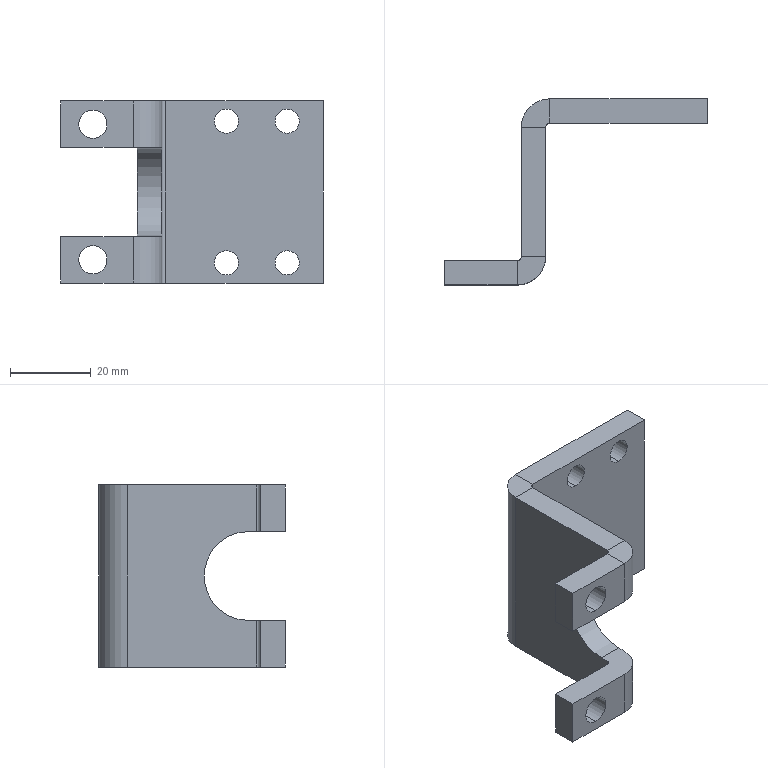Part | SolidWorks | features ICE 3, FlatPattern 1, SMBaseFlange 1, SheetMetal 1 | 1 solid | 42 faces | box 65 x 46 x 45 mm | volume 21673 mm3 | plane 23 | cylinder 19 | commonest cylinder face diameters 6 x8 7 x4 2 x3 14 x3 22 x1
STEP:
#1=CARTESIAN_POINT('',(8.,0.,2.25));
#2=VERTEX_POINT('',#1);
#3=CARTESIAN_POINT('',(8.,0.,9.25));
#4=VERTEX_POINT('',#3);
#5=CARTESIAN_POINT('',(8.,0.,5.75));
#6=DIRECTION('',(0.,1.,0.));
#7=DIRECTION('',(0.,0.,1.));
#8=AXIS2_PLACEMENT_3D('',#5,#6,#7);
#9=CIRCLE('',#8,3.5);
#10=EDGE_CURVE('',#2,#4,#9,.T.);
#11=ORIENTED_EDGE('',*,*,#10,.F.);
#12=CARTESIAN_POINT('',(8.,6.,2.25));
#13=VERTEX_POINT('',#12);
#14=CARTESIAN_POINT('',(8.,-4.,2.25));
#15=DIRECTION('',(0.,1.,0.));
#16=VECTOR('',#15,1000.);
#17=LINE('',#14,#16);
#18=EDGE_CURVE('',#2,#13,#17,.T.);
#19=ORIENTED_EDGE('',*,*,#18,.T.);
#20=CARTESIAN_POINT('',(8.,6.,9.25));
#21=VERTEX_POINT('',#20);
#22=CARTESIAN_POINT('',(8.,6.,5.75));
#23=DIRECTION('',(0.,1.,0.));
#24=DIRECTION('',(0.,0.,1.));
#25=AXIS2_PLACEMENT_3D('',#22,#23,#24);
#26=CIRCLE('',#25,3.5);
#27=EDGE_CURVE('',#13,#21,#26,.T.);
#28=ORIENTED_EDGE('',*,*,#27,.T.);
#29=CARTESIAN_POINT('',(8.,-4.,9.25));
#30=DIRECTION('',(0.,1.,0.));
#31=VECTOR('',#30,1000.);
#32=LINE('',#29,#31);
#33=EDGE_CURVE('',#4,#21,#32,.T.);
#34=ORIENTED_EDGE('',*,*,#33,.F.);
#35=EDGE_LOOP('',(#11,#19,#28,#34));
#36=FACE_OUTER_BOUND('',#35,.T.);
#37=CARTESIAN_POINT('',(8.,-4.,5.75));
#38=DIRECTION('',(0.,1.,0.));
#39=DIRECTION('',(0.,0.,1.));
#40=AXIS2_PLACEMENT_3D('',#37,#38,#39);
#41=CYLINDRICAL_SURFACE('',#40,3.5);
#42=ADVANCED_FACE('',(#36),#41,.F.);
#43=CARTESIAN_POINT('',(8.,0.,35.75));
#44=VERTEX_POINT('',#43);
#45=CARTESIAN_POINT('',(8.,0.,42.75));
#46=VERTEX_POINT('',#45);
#47=CARTESIAN_POINT('',(8.,0.,39.25));
#48=DIRECTION('',(0.,1.,0.));
#49=DIRECTION('',(0.,0.,1.));
#50=AXIS2_PLACEMENT_3D('',#47,#48,#49);
#51=CIRCLE('',#50,3.5);
#52=EDGE_CURVE('',#44,#46,#51,.T.);
#53=ORIENTED_EDGE('',*,*,#52,.F.);
#54=CARTESIAN_POINT('',(8.,6.,35.75));
#55=VERTEX_POINT('',#54);
#56=CARTESIAN_POINT('',(8.,-4.,35.75));
#57=DIRECTION('',(0.,1.,0.));
#58=VECTOR('',#57,1000.);
#59=LINE('',#56,#58);
#60=EDGE_CURVE('',#44,#55,#59,.T.);
#61=ORIENTED_EDGE('',*,*,#60,.T.);
#62=CARTESIAN_POINT('',(8.,6.,42.75));
#63=VERTEX_POINT('',#62);
#64=CARTESIAN_POINT('',(8.,6.,39.25));
#65=DIRECTION('',(0.,1.,0.));
#66=DIRECTION('',(0.,0.,1.));
#67=AXIS2_PLACEMENT_3D('',#64,#65,#66);
#68=CIRCLE('',#67,3.5);
#69=EDGE_CURVE('',#55,#63,#68,.T.);
#70=ORIENTED_EDGE('',*,*,#69,.T.);
#71=CARTESIAN_POINT('',(8.,-4.,42.75));
#72=DIRECTION('',(0.,1.,0.));
#73=VECTOR('',#72,1000.);
#74=LINE('',#71,#73);
#75=EDGE_CURVE('',#46,#63,#74,.T.);
#76=ORIENTED_EDGE('',*,*,#75,.F.);
#77=EDGE_LOOP('',(#53,#61,#70,#76));
#78=FACE_OUTER_BOUND('',#77,.T.);
#79=CARTESIAN_POINT('',(8.,-4.,39.25));
#80=DIRECTION('',(0.,1.,0.));
#81=DIRECTION('',(0.,0.,1.));
#82=AXIS2_PLACEMENT_3D('',#79,#80,#81);
#83=CYLINDRICAL_SURFACE('',#82,3.5);
#84=ADVANCED_FACE('',(#78),#83,.F.);
#85=CARTESIAN_POINT('',(56.,40.,2.));
#86=VERTEX_POINT('',#85);
#87=CARTESIAN_POINT('',(56.,40.,8.));
#88=VERTEX_POINT('',#87);
#89=CARTESIAN_POINT('',(56.,40.,5.));
#90=DIRECTION('',(0.,1.,0.));
#91=DIRECTION('',(0.,0.,1.));
#92=AXIS2_PLACEMENT_3D('',#89,#90,#91);
#93=CIRCLE('',#92,3.);
#94=EDGE_CURVE('',#86,#88,#93,.T.);
#95=ORIENTED_EDGE('',*,*,#94,.F.);
#96=CARTESIAN_POINT('',(56.,46.,2.));
#97=VERTEX_POINT('',#96);
#98=CARTESIAN_POINT('',(56.,36.,2.));
#99=DIRECTION('',(0.,1.,0.));
#100=VECTOR('',#99,1000.);
#101=LINE('',#98,#100);
#102=EDGE_CURVE('',#86,#97,#101,.T.);
#103=ORIENTED_EDGE('',*,*,#102,.T.);
#104=CARTESIAN_POINT('',(56.,46.,8.));
#105=VERTEX_POINT('',#104);
#106=CARTESIAN_POINT('',(56.,46.,5.));
#107=DIRECTION('',(0.,1.,0.));
#108=DIRECTION('',(0.,0.,1.));
#109=AXIS2_PLACEMENT_3D('',#106,#107,#108);
#110=CIRCLE('',#109,3.);
#111=EDGE_CURVE('',#97,#105,#110,.T.);
#112=ORIENTED_EDGE('',*,*,#111,.T.);
#113=CARTESIAN_POINT('',(56.,36.,8.));
#114=DIRECTION('',(0.,1.,0.));
#115=VECTOR('',#114,1000.);
#116=LINE('',#113,#115);
#117=EDGE_CURVE('',#88,#105,#116,.T.);
#118=ORIENTED_EDGE('',*,*,#117,.F.);
#119=EDGE_LOOP('',(#95,#103,#112,#118));
#120=FACE_OUTER_BOUND('',#119,.T.);
#121=CARTESIAN_POINT('',(56.,36.,5.));
#122=DIRECTION('',(0.,1.,0.));
#123=DIRECTION('',(0.,0.,1.));
#124=AXIS2_PLACEMENT_3D('',#121,#122,#123);
#125=CYLINDRICAL_SURFACE('',#124,3.);
#126=ADVANCED_FACE('',(#120),#125,.F.);
#127=CARTESIAN_POINT('',(56.,40.,37.));
#128=VERTEX_POINT('',#127);
#129=CARTESIAN_POINT('',(56.,40.,43.));
#130=VERTEX_POINT('',#129);
#131=CARTESIAN_POINT('',(56.,40.,40.));
#132=DIRECTION('',(0.,1.,0.));
#133=DIRECTION('',(0.,0.,1.));
#134=AXIS2_PLACEMENT_3D('',#131,#132,#133);
#135=CIRCLE('',#134,3.);
#136=EDGE_CURVE('',#128,#130,#135,.T.);
#137=ORIENTED_EDGE('',*,*,#136,.F.);
#138=CARTESIAN_POINT('',(56.,46.,37.));
#139=VERTEX_POINT('',#138);
#140=CARTESIAN_POINT('',(56.,36.,37.));
#141=DIRECTION('',(0.,1.,0.));
#142=VECTOR('',#141,1000.);
#143=LINE('',#140,#142);
#144=EDGE_CURVE('',#128,#139,#143,.T.);
#145=ORIENTED_EDGE('',*,*,#144,.T.);
#146=CARTESIAN_POINT('',(56.,46.,43.));
#147=VERTEX_POINT('',#146);
#148=CARTESIAN_POINT('',(56.,46.,40.));
#149=DIRECTION('',(0.,1.,0.));
#150=DIRECTION('',(0.,0.,1.));
#151=AXIS2_PLACEMENT_3D('',#148,#149,#150);
#152=CIRCLE('',#151,3.);
#153=EDGE_CURVE('',#139,#147,#152,.T.);
#154=ORIENTED_EDGE('',*,*,#153,.T.);
#155=CARTESIAN_POINT('',(56.,36.,43.));
#156=DIRECTION('',(0.,1.,0.));
#157=VECTOR('',#156,1000.);
#158=LINE('',#155,#157);
#159=EDGE_CURVE('',#130,#147,#158,.T.);
#160=ORIENTED_EDGE('',*,*,#159,.F.);
#161=EDGE_LOOP('',(#137,#145,#154,#160));
#162=FACE_OUTER_BOUND('',#161,.T.);
#163=CARTESIAN_POINT('',(56.,36.,40.));
#164=DIRECTION('',(0.,1.,0.));
#165=DIRECTION('',(0.,0.,1.));
#166=AXIS2_PLACEMENT_3D('',#163,#164,#165);
#167=CYLINDRICAL_SURFACE('',#166,3.);
#168=ADVANCED_FACE('',(#162),#167,.F.);
#169=CARTESIAN_POINT('',(41.,40.,37.));
#170=VERTEX_POINT('',#169);
#171=CARTESIAN_POINT('',(41.,40.,43.));
#172=VERTEX_POINT('',#171);
#173=CARTESIAN_POINT('',(41.,40.,40.));
#174=DIRECTION('',(0.,1.,0.));
#175=DIRECTION('',(0.,0.,1.));
#176=AXIS2_PLACEMENT_3D('',#173,#174,#175);
#177=CIRCLE('',#176,3.);
#178=EDGE_CURVE('',#170,#172,#177,.T.);
#179=ORIENTED_EDGE('',*,*,#178,.F.);
#180=CARTESIAN_POINT('',(41.,46.,37.));
#181=VERTEX_POINT('',#180);
#182=CARTESIAN_POINT('',(41.,36.,37.));
#183=DIRECTION('',(0.,1.,0.));
#184=VECTOR('',#183,1000.);
#185=LINE('',#182,#184);
#186=EDGE_CURVE('',#170,#181,#185,.T.);
#187=ORIENTED_EDGE('',*,*,#186,.T.);
#188=CARTESIAN_POINT('',(41.,46.,43.));
#189=VERTEX_POINT('',#188);
#190=CARTESIAN_POINT('',(41.,46.,40.));
#191=DIRECTION('',(0.,1.,0.));
#192=DIRECTION('',(0.,0.,1.));
#193=AXIS2_PLACEMENT_3D('',#190,#191,#192);
#194=CIRCLE('',#193,3.);
#195=EDGE_CURVE('',#181,#189,#194,.T.);
#196=ORIENTED_EDGE('',*,*,#195,.T.);
#197=CARTESIAN_POINT('',(41.,36.,43.));
#198=DIRECTION('',(0.,1.,0.));
#199=VECTOR('',#198,1000.);
#200=LINE('',#197,#199);
#201=EDGE_CURVE('',#172,#189,#200,.T.);
#202=ORIENTED_EDGE('',*,*,#201,.F.);
#203=EDGE_LOOP('',(#179,#187,#196,#202));
#204=FACE_OUTER_BOUND('',#203,.T.);
#205=CARTESIAN_POINT('',(41.,36.,40.));
#206=DIRECTION('',(0.,1.,0.));
#207=DIRECTION('',(0.,0.,1.));
#208=AXIS2_PLACEMENT_3D('',#205,#206,#207);
#209=CYLINDRICAL_SURFACE('',#208,3.);
#210=ADVANCED_FACE('',(#204),#209,.F.);
#211=CARTESIAN_POINT('',(41.,40.,2.));
#212=VERTEX_POINT('',#211);
#213=CARTESIAN_POINT('',(41.,40.,8.));
#214=VERTEX_POINT('',#213);
#215=CARTESIAN_POINT('',(41.,40.,5.));
#216=DIRECTION('',(0.,1.,0.));
#217=DIRECTION('',(0.,0.,1.));
#218=AXIS2_PLACEMENT_3D('',#215,#216,#217);
#219=CIRCLE('',#218,3.);
#220=EDGE_CURVE('',#212,#214,#219,.T.);
#221=ORIENTED_EDGE('',*,*,#220,.F.);
#222=CARTESIAN_POINT('',(41.,46.,2.));
#223=VERTEX_POINT('',#222);
#224=CARTESIAN_POINT('',(41.,36.,2.));
#225=DIRECTION('',(0.,1.,0.));
#226=VECTOR('',#225,1000.);
#227=LINE('',#224,#226);
#228=EDGE_CURVE('',#212,#223,#227,.T.);
#229=ORIENTED_EDGE('',*,*,#228,.T.);
#230=CARTESIAN_POINT('',(41.,46.,8.));
#231=VERTEX_POINT('',#230);
#232=CARTESIAN_POINT('',(41.,46.,5.));
#233=DIRECTION('',(0.,1.,0.));
#234=DIRECTION('',(0.,0.,1.));
#235=AXIS2_PLACEMENT_3D('',#232,#233,#234);
#236=CIRCLE('',#235,3.);
#237=EDGE_CURVE('',#223,#231,#236,.T.);
#238=ORIENTED_EDGE('',*,*,#237,.T.);
#239=CARTESIAN_POINT('',(41.,36.,8.));
#240=DIRECTION('',(0.,1.,0.));
#241=VECTOR('',#240,1000.);
#242=LINE('',#239,#241);
#243=EDGE_CURVE('',#214,#231,#242,.T.);
#244=ORIENTED_EDGE('',*,*,#243,.F.);
#245=EDGE_LOOP('',(#221,#229,#238,#244));
#246=FACE_OUTER_BOUND('',#245,.T.);
#247=CARTESIAN_POINT('',(41.,36.,5.));
#248=DIRECTION('',(0.,1.,0.));
#249=DIRECTION('',(0.,0.,1.));
#250=AXIS2_PLACEMENT_3D('',#247,#248,#249);
#251=CYLINDRICAL_SURFACE('',#250,3.);
#252=ADVANCED_FACE('',(#246),#251,.F.);
#253=CARTESIAN_POINT('',(19.,7.,11.5));
#254=VERTEX_POINT('',#253);
#255=CARTESIAN_POINT('',(18.,6.,11.5));
#256=VERTEX_POINT('',#255);
#257=CARTESIAN_POINT('',(18.,7.,11.5));
#258=DIRECTION('',(0.,0.,-1.));
#259=DIRECTION('',(-1.,0.,0.));
#260=AXIS2_PLACEMENT_3D('',#257,#258,#259);
#261=CIRCLE('',#260,1.);
#262=EDGE_CURVE('',#254,#256,#261,.T.);
#263=ORIENTED_EDGE('',*,*,#262,.F.);
#264=CARTESIAN_POINT('',(19.,7.,0.));
#265=VERTEX_POINT('',#264);
#266=CARTESIAN_POINT('',(19.,7.,45.));
#267=DIRECTION('',(0.,0.,-1.));
#268=VECTOR('',#267,1000.);
#269=LINE('',#266,#268);
#270=EDGE_CURVE('',#254,#265,#269,.T.);
#271=ORIENTED_EDGE('',*,*,#270,.T.);
#272=CARTESIAN_POINT('',(18.,6.,0.));
#273=VERTEX_POINT('',#272);
#274=CARTESIAN_POINT('',(18.,7.,0.));
#275=DIRECTION('',(0.,0.,1.));
#276=DIRECTION('',(1.,0.,0.));
#277=AXIS2_PLACEMENT_3D('',#274,#275,#276);
#278=CIRCLE('',#277,1.);
#279=EDGE_CURVE('',#273,#265,#278,.T.);
#280=ORIENTED_EDGE('',*,*,#279,.F.);
#281=CARTESIAN_POINT('',(18.,6.,45.));
#282=DIRECTION('',(0.,0.,-1.));
#283=VECTOR('',#282,1000.);
#284=LINE('',#281,#283);
#285=EDGE_CURVE('',#256,#273,#284,.T.);
#286=ORIENTED_EDGE('',*,*,#285,.F.);
#287=EDGE_LOOP('',(#263,#271,#280,#286));
#288=FACE_OUTER_BOUND('',#287,.T.);
#289=CARTESIAN_POINT('',(18.,7.,45.));
#290=DIRECTION('',(0.,0.,-1.));
#291=DIRECTION('',(-1.,0.,0.));
#292=AXIS2_PLACEMENT_3D('',#289,#290,#291);
#293=CYLINDRICAL_SURFACE('',#292,1.);
#294=ADVANCED_FACE('',(#288),#293,.F.);
#295=CARTESIAN_POINT('',(8.,6.,5.75));
#296=DIRECTION('',(0.,1.,0.));
#297=DIRECTION('',(0.,0.,1.));
#298=AXIS2_PLACEMENT_3D('',#295,#296,#297);
#299=CIRCLE('',#298,3.5);
#300=EDGE_CURVE('',#21,#13,#299,.T.);
#301=ORIENTED_EDGE('',*,*,#300,.F.);
#302=ORIENTED_EDGE('',*,*,#27,.F.);
#303=EDGE_LOOP('',(#301,#302));
#304=FACE_BOUND('',#303,.T.);
#305=CARTESIAN_POINT('',(0.,6.,11.5));
#306=VERTEX_POINT('',#305);
#307=CARTESIAN_POINT('',(0.,6.,11.5));
#308=DIRECTION('',(-1.,0.,0.));
#309=VECTOR('',#308,1000.);
#310=LINE('',#307,#309);
#311=EDGE_CURVE('',#256,#306,#310,.T.);
#312=ORIENTED_EDGE('',*,*,#311,.F.);
#313=ORIENTED_EDGE('',*,*,#285,.T.);
#314=CARTESIAN_POINT('',(0.,6.,0.));
#315=VERTEX_POINT('',#314);
#316=CARTESIAN_POINT('',(0.,6.,0.));
#317=DIRECTION('',(1.,0.,0.));
#318=VECTOR('',#317,1000.);
#319=LINE('',#316,#318);
#320=EDGE_CURVE('',#315,#273,#319,.T.);
#321=ORIENTED_EDGE('',*,*,#320,.F.);
#322=CARTESIAN_POINT('',(0.,6.,45.));
#323=DIRECTION('',(0.,0.,-1.));
#324=VECTOR('',#323,1000.);
#325=LINE('',#322,#324);
#326=EDGE_CURVE('',#306,#315,#325,.T.);
#327=ORIENTED_EDGE('',*,*,#326,.F.);
#328=EDGE_LOOP('',(#312,#313,#321,#327));
#329=FACE_OUTER_BOUND('',#328,.T.);
#330=CARTESIAN_POINT('',(0.,6.,45.));
#331=DIRECTION('',(0.,1.,0.));
#332=DIRECTION('',(0.,0.,1.));
#333=AXIS2_PLACEMENT_3D('',#330,#331,#332);
#334=PLANE('',#333);
#335=ADVANCED_FACE('',(#304,#329),#334,.T.);
#336=CARTESIAN_POINT('',(0.,0.,11.5));
#337=VERTEX_POINT('',#336);
#338=CARTESIAN_POINT('',(0.,-9.188,11.5));
#339=DIRECTION('',(0.,-1.,0.));
#340=VECTOR('',#339,1000.);
#341=LINE('',#338,#340);
#342=EDGE_CURVE('',#306,#337,#341,.T.);
#343=ORIENTED_EDGE('',*,*,#342,.F.);
#344=ORIENTED_EDGE('',*,*,#326,.T.);
#345=CARTESIAN_POINT('',(0.,0.,0.));
#346=VERTEX_POINT('',#345);
#347=CARTESIAN_POINT('',(0.,0.,0.));
#348=DIRECTION('',(0.,1.,0.));
#349=VECTOR('',#348,1000.);
#350=LINE('',#347,#349);
#351=EDGE_CURVE('',#346,#315,#350,.T.);
#352=ORIENTED_EDGE('',*,*,#351,.F.);
#353=CARTESIAN_POINT('',(0.,0.,45.));
#354=DIRECTION('',(0.,0.,-1.));
#355=VECTOR('',#354,1000.);
#356=LINE('',#353,#355);
#357=EDGE_CURVE('',#337,#346,#356,.T.);
#358=ORIENTED_EDGE('',*,*,#357,.F.);
#359=EDGE_LOOP('',(#343,#344,#352,#358));
#360=FACE_OUTER_BOUND('',#359,.T.);
#361=CARTESIAN_POINT('',(0.,0.,45.));
#362=DIRECTION('',(-1.,0.,0.));
#363=DIRECTION('',(0.,0.,1.));
#364=AXIS2_PLACEMENT_3D('',#361,#362,#363);
#365=PLANE('',#364);
#366=ADVANCED_FACE('',(#360),#365,.T.);
#367=CARTESIAN_POINT('',(8.,0.,5.75));
#368=DIRECTION('',(0.,1.,0.));
#369=DIRECTION('',(0.,0.,1.));
#370=AXIS2_PLACEMENT_3D('',#367,#368,#369);
#371=CIRCLE('',#370,3.5);
#372=EDGE_CURVE('',#4,#2,#371,.T.);
#373=ORIENTED_EDGE('',*,*,#372,.T.);
#374=ORIENTED_EDGE('',*,*,#10,.T.);
#375=EDGE_LOOP('',(#373,#374));
#376=FACE_BOUND('',#375,.T.);
#377=CARTESIAN_POINT('',(18.,0.,11.5));
#378=VERTEX_POINT('',#377);
#379=CARTESIAN_POINT('',(18.,0.,0.));
#380=VERTEX_POINT('',#379);
#381=CARTESIAN_POINT('',(18.,0.,45.));
#382=DIRECTION('',(0.,0.,-1.));
#383=VECTOR('',#382,1000.);
#384=LINE('',#381,#383);
#385=EDGE_CURVE('',#378,#380,#384,.T.);
#386=ORIENTED_EDGE('',*,*,#385,.F.);
#387=CARTESIAN_POINT('',(0.,0.,11.5));
#388=DIRECTION('',(-1.,0.,0.));
#389=VECTOR('',#388,1000.);
#390=LINE('',#387,#389);
#391=EDGE_CURVE('',#378,#337,#390,.T.);
#392=ORIENTED_EDGE('',*,*,#391,.T.);
#393=ORIENTED_EDGE('',*,*,#357,.T.);
#394=CARTESIAN_POINT('',(0.,0.,0.));
#395=DIRECTION('',(1.,0.,0.));
#396=VECTOR('',#395,1000.);
#397=LINE('',#394,#396);
#398=EDGE_CURVE('',#346,#380,#397,.T.);
#399=ORIENTED_EDGE('',*,*,#398,.T.);
#400=EDGE_LOOP('',(#386,#392,#393,#399));
#401=FACE_OUTER_BOUND('',#400,.T.);
#402=CARTESIAN_POINT('',(0.,0.,45.));
#403=DIRECTION('',(0.,1.,0.));
#404=DIRECTION('',(0.,0.,1.));
#405=AXIS2_PLACEMENT_3D('',#402,#403,#404);
#406=PLANE('',#405);
#407=ADVANCED_FACE('',(#376,#401),#406,.F.);
#408=CARTESIAN_POINT('',(25.,7.,11.5));
#409=VERTEX_POINT('',#408);
#410=CARTESIAN_POINT('',(25.,7.,0.));
#411=VERTEX_POINT('',#410);
#412=CARTESIAN_POINT('',(25.,7.,45.));
#413=DIRECTION('',(0.,0.,-1.));
#414=VECTOR('',#413,1000.);
#415=LINE('',#412,#414);
#416=EDGE_CURVE('',#409,#411,#415,.T.);
#417=ORIENTED_EDGE('',*,*,#416,.F.);
#418=CARTESIAN_POINT('',(18.,7.,11.5));
#419=DIRECTION('',(0.,0.,-1.));
#420=DIRECTION('',(-1.,0.,0.));
#421=AXIS2_PLACEMENT_3D('',#418,#419,#420);
#422=CIRCLE('',#421,7.);
#423=EDGE_CURVE('',#409,#378,#422,.T.);
#424=ORIENTED_EDGE('',*,*,#423,.T.);
#425=ORIENTED_EDGE('',*,*,#385,.T.);
#426=CARTESIAN_POINT('',(18.,7.,0.));
#427=DIRECTION('',(0.,0.,1.));
#428=DIRECTION('',(-1.,0.,0.));
#429=AXIS2_PLACEMENT_3D('',#426,#427,#428);
#430=CIRCLE('',#429,7.);
#431=EDGE_CURVE('',#380,#411,#430,.T.);
#432=ORIENTED_EDGE('',*,*,#431,.T.);
#433=EDGE_LOOP('',(#417,#424,#425,#432));
#434=FACE_OUTER_BOUND('',#433,.T.);
#435=CARTESIAN_POINT('',(18.,7.,45.));
#436=DIRECTION('',(0.,0.,-1.));
#437=DIRECTION('',(-1.,0.,0.));
#438=AXIS2_PLACEMENT_3D('',#435,#436,#437);
#439=CYLINDRICAL_SURFACE('',#438,7.);
#440=ADVANCED_FACE('',(#434),#439,.T.);
#441=CARTESIAN_POINT('',(18.,0.,45.));
#442=VERTEX_POINT('',#441);
#443=CARTESIAN_POINT('',(18.,6.,45.));
#444=VERTEX_POINT('',#443);
#445=CARTESIAN_POINT('',(18.,0.,45.));
#446=DIRECTION('',(0.,1.,0.));
#447=VECTOR('',#446,1000.);
#448=LINE('',#445,#447);
#449=EDGE_CURVE('',#442,#444,#448,.T.);
#450=ORIENTED_EDGE('',*,*,#449,.F.);
#451=CARTESIAN_POINT('',(25.,7.,45.));
#452=VERTEX_POINT('',#451);
#453=CARTESIAN_POINT('',(18.,7.,45.));
#454=DIRECTION('',(0.,0.,1.));
#455=DIRECTION('',(-1.,0.,0.));
#456=AXIS2_PLACEMENT_3D('',#453,#454,#455);
#457=CIRCLE('',#456,7.);
#458=EDGE_CURVE('',#442,#452,#457,.T.);
#459=ORIENTED_EDGE('',*,*,#458,.T.);
#460=CARTESIAN_POINT('',(19.,7.,45.));
#461=VERTEX_POINT('',#460);
#462=CARTESIAN_POINT('',(19.,7.,45.));
#463=DIRECTION('',(1.,0.,0.));
#464=VECTOR('',#463,1000.);
#465=LINE('',#462,#464);
#466=EDGE_CURVE('',#461,#452,#465,.T.);
#467=ORIENTED_EDGE('',*,*,#466,.F.);
#468=CARTESIAN_POINT('',(18.,7.,45.));
#469=DIRECTION('',(0.,0.,1.));
#470=DIRECTION('',(1.,0.,0.));
#471=AXIS2_PLACEMENT_3D('',#468,#469,#470);
#472=CIRCLE('',#471,1.);
#473=EDGE_CURVE('',#444,#461,#472,.T.);
#474=ORIENTED_EDGE('',*,*,#473,.F.);
#475=EDGE_LOOP('',(#450,#459,#467,#474));
#476=FACE_OUTER_BOUND('',#475,.T.);
#477=CARTESIAN_POINT('',(18.,0.,45.));
#478=DIRECTION('',(0.,0.,1.));
#479=DIRECTION('',(1.,0.,0.));
#480=AXIS2_PLACEMENT_3D('',#477,#478,#479);
#481=PLANE('',#480);
#482=ADVANCED_FACE('',(#476),#481,.T.);
#483=CARTESIAN_POINT('',(0.,0.,45.));
#484=VERTEX_POINT('',#483);
#485=CARTESIAN_POINT('',(0.,0.,45.));
#486=DIRECTION('',(1.,0.,0.));
#487=VECTOR('',#486,1000.);
#488=LINE('',#485,#487);
#489=EDGE_CURVE('',#484,#442,#488,.T.);
#490=ORIENTED_EDGE('',*,*,#489,.T.);
#491=ORIENTED_EDGE('',*,*,#449,.T.);
#492=CARTESIAN_POINT('',(0.,6.,45.));
#493=VERTEX_POINT('',#492);
#494=CARTESIAN_POINT('',(0.,6.,45.));
#495=DIRECTION('',(1.,0.,0.));
#496=VECTOR('',#495,1000.);
#497=LINE('',#494,#496);
#498=EDGE_CURVE('',#493,#444,#497,.T.);
#499=ORIENTED_EDGE('',*,*,#498,.F.);
#500=CARTESIAN_POINT('',(0.,0.,45.));
#501=DIRECTION('',(0.,1.,0.));
#502=VECTOR('',#501,1000.);
#503=LINE('',#500,#502);
#504=EDGE_CURVE('',#484,#493,#503,.T.);
#505=ORIENTED_EDGE('',*,*,#504,.F.);
#506=EDGE_LOOP('',(#490,#491,#499,#505));
#507=FACE_OUTER_BOUND('',#506,.T.);
#508=CARTESIAN_POINT('',(19.,7.,45.));
#509=DIRECTION('',(0.,0.,1.));
#510=DIRECTION('',(1.,0.,0.));
#511=AXIS2_PLACEMENT_3D('',#508,#509,#510);
#512=PLANE('',#511);
#513=ADVANCED_FACE('',(#507),#512,.T.);
#514=CARTESIAN_POINT('',(25.,7.,0.));
#515=DIRECTION('',(-1.,0.,0.));
#516=VECTOR('',#515,1000.);
#517=LINE('',#514,#516);
#518=EDGE_CURVE('',#411,#265,#517,.T.);
#519=ORIENTED_EDGE('',*,*,#518,.F.);
#520=ORIENTED_EDGE('',*,*,#431,.F.);
#521=CARTESIAN_POINT('',(18.,6.,0.));
#522=DIRECTION('',(0.,-1.,0.));
#523=VECTOR('',#522,1000.);
#524=LINE('',#521,#523);
#525=EDGE_CURVE('',#273,#380,#524,.T.);
#526=ORIENTED_EDGE('',*,*,#525,.F.);
#527=ORIENTED_EDGE('',*,*,#279,.T.);
#528=EDGE_LOOP('',(#519,#520,#526,#527));
#529=FACE_OUTER_BOUND('',#528,.T.);
#530=CARTESIAN_POINT('',(25.,7.,0.));
#531=DIRECTION('',(0.,0.,-1.));
#532=DIRECTION('',(-1.,0.,0.));
#533=AXIS2_PLACEMENT_3D('',#530,#531,#532);
#534=PLANE('',#533);
#535=ADVANCED_FACE('',(#529),#534,.T.);
#536=CARTESIAN_POINT('',(25.,39.,0.));
#537=VERTEX_POINT('',#536);
#538=CARTESIAN_POINT('',(25.,0.,0.));
#539=DIRECTION('',(0.,1.,0.));
#540=VECTOR('',#539,1000.);
#541=LINE('',#538,#540);
#542=EDGE_CURVE('',#411,#537,#541,.T.);
#543=ORIENTED_EDGE('',*,*,#542,.F.);
#544=ORIENTED_EDGE('',*,*,#518,.T.);
#545=CARTESIAN_POINT('',(19.,39.,0.));
#546=VERTEX_POINT('',#545);
#547=CARTESIAN_POINT('',(19.,0.,0.));
#548=DIRECTION('',(0.,1.,0.));
#549=VECTOR('',#548,1000.);
#550=LINE('',#547,#549);
#551=EDGE_CURVE('',#265,#546,#550,.T.);
#552=ORIENTED_EDGE('',*,*,#551,.T.);
#553=CARTESIAN_POINT('',(19.,39.,0.));
#554=DIRECTION('',(1.,0.,0.));
#555=VECTOR('',#554,1000.);
#556=LINE('',#553,#555);
#557=EDGE_CURVE('',#546,#537,#556,.T.);
#558=ORIENTED_EDGE('',*,*,#557,.T.);
#559=EDGE_LOOP('',(#543,#544,#552,#558));
#560=FACE_OUTER_BOUND('',#559,.T.);
#561=CARTESIAN_POINT('',(18.,6.,0.));
#562=DIRECTION('',(0.,0.,-1.));
#563=DIRECTION('',(-1.,0.,0.));
#564=AXIS2_PLACEMENT_3D('',#561,#562,#563);
#565=PLANE('',#564);
#566=ADVANCED_FACE('',(#560),#565,.T.);
#567=CARTESIAN_POINT('',(25.,39.,45.));
#568=VERTEX_POINT('',#567);
#569=CARTESIAN_POINT('',(19.,39.,45.));
#570=VERTEX_POINT('',#569);
#571=CARTESIAN_POINT('',(25.,39.,45.));
#572=DIRECTION('',(-1.,0.,0.));
#573=VECTOR('',#572,1000.);
#574=LINE('',#571,#573);
#575=EDGE_CURVE('',#568,#570,#574,.T.);
#576=ORIENTED_EDGE('',*,*,#575,.F.);
#577=CARTESIAN_POINT('',(26.,40.,45.));
#578=VERTEX_POINT('',#577);
#579=CARTESIAN_POINT('',(26.,39.,45.));
#580=DIRECTION('',(0.,0.,-1.));
#581=DIRECTION('',(1.,0.,0.));
#582=AXIS2_PLACEMENT_3D('',#579,#580,#581);
#583=CIRCLE('',#582,1.);
#584=EDGE_CURVE('',#568,#578,#583,.T.);
#585=ORIENTED_EDGE('',*,*,#584,.T.);
#586=CARTESIAN_POINT('',(26.,46.,45.));
#587=VERTEX_POINT('',#586);
#588=CARTESIAN_POINT('',(26.,46.,45.));
#589=DIRECTION('',(0.,-1.,0.));
#590=VECTOR('',#589,1000.);
#591=LINE('',#588,#590);
#592=EDGE_CURVE('',#587,#578,#591,.T.);
#593=ORIENTED_EDGE('',*,*,#592,.F.);
#594=CARTESIAN_POINT('',(26.,39.,45.));
#595=DIRECTION('',(0.,0.,-1.));
#596=DIRECTION('',(1.,0.,0.));
#597=AXIS2_PLACEMENT_3D('',#594,#595,#596);
#598=CIRCLE('',#597,7.);
#599=EDGE_CURVE('',#570,#587,#598,.T.);
#600=ORIENTED_EDGE('',*,*,#599,.F.);
#601=EDGE_LOOP('',(#576,#585,#593,#600));
#602=FACE_OUTER_BOUND('',#601,.T.);
#603=CARTESIAN_POINT('',(25.,39.,45.));
#604=DIRECTION('',(0.,0.,1.));
#605=DIRECTION('',(1.,0.,0.));
#606=AXIS2_PLACEMENT_3D('',#603,#604,#605);
#607=PLANE('',#606);
#608=ADVANCED_FACE('',(#602),#607,.T.);
#609=CARTESIAN_POINT('',(25.,0.,45.));
#610=DIRECTION('',(0.,1.,0.));
#611=VECTOR('',#610,1000.);
#612=LINE('',#609,#611);
#613=EDGE_CURVE('',#452,#568,#612,.T.);
#614=ORIENTED_EDGE('',*,*,#613,.T.);
#615=ORIENTED_EDGE('',*,*,#575,.T.);
#616=CARTESIAN_POINT('',(19.,0.,45.));
#617=DIRECTION('',(0.,1.,0.));
#618=VECTOR('',#617,1000.);
#619=LINE('',#616,#618);
#620=EDGE_CURVE('',#461,#570,#619,.T.);
#621=ORIENTED_EDGE('',*,*,#620,.F.);
#622=ORIENTED_EDGE('',*,*,#466,.T.);
#623=EDGE_LOOP('',(#614,#615,#621,#622));
#624=FACE_OUTER_BOUND('',#623,.T.);
#625=CARTESIAN_POINT('',(26.,46.,45.));
#626=DIRECTION('',(0.,0.,1.));
#627=DIRECTION('',(1.,0.,0.));
#628=AXIS2_PLACEMENT_3D('',#625,#626,#627);
#629=PLANE('',#628);
#630=ADVANCED_FACE('',(#624),#629,.T.);
#631=CARTESIAN_POINT('',(26.,40.,0.));
#632=VERTEX_POINT('',#631);
#633=CARTESIAN_POINT('',(26.,46.,0.));
#634=VERTEX_POINT('',#633);
#635=CARTESIAN_POINT('',(26.,40.,0.));
#636=DIRECTION('',(0.,1.,0.));
#637=VECTOR('',#636,1000.);
#638=LINE('',#635,#637);
#639=EDGE_CURVE('',#632,#634,#638,.T.);
#640=ORIENTED_EDGE('',*,*,#639,.F.);
#641=CARTESIAN_POINT('',(26.,39.,0.));
#642=DIRECTION('',(0.,0.,-1.));
#643=DIRECTION('',(1.,0.,0.));
#644=AXIS2_PLACEMENT_3D('',#641,#642,#643);
#645=CIRCLE('',#644,1.);
#646=EDGE_CURVE('',#537,#632,#645,.T.);
#647=ORIENTED_EDGE('',*,*,#646,.F.);
#648=ORIENTED_EDGE('',*,*,#557,.F.);
#649=CARTESIAN_POINT('',(26.,39.,0.));
#650=DIRECTION('',(0.,0.,-1.));
#651=DIRECTION('',(1.,0.,0.));
#652=AXIS2_PLACEMENT_3D('',#649,#650,#651);
#653=CIRCLE('',#652,7.);
#654=EDGE_CURVE('',#546,#634,#653,.T.);
#655=ORIENTED_EDGE('',*,*,#654,.T.);
#656=EDGE_LOOP('',(#640,#647,#648,#655));
#657=FACE_OUTER_BOUND('',#656,.T.);
#658=CARTESIAN_POINT('',(26.,40.,0.));
#659=DIRECTION('',(0.,0.,-1.));
#660=DIRECTION('',(-1.,0.,0.));
#661=AXIS2_PLACEMENT_3D('',#658,#659,#660);
#662=PLANE('',#661);
#663=ADVANCED_FACE('',(#657),#662,.T.);
#664=CARTESIAN_POINT('',(65.,40.,0.));
#665=VERTEX_POINT('',#664);
#666=CARTESIAN_POINT('',(25.,40.,0.));
#667=DIRECTION('',(1.,0.,0.));
#668=VECTOR('',#667,1000.);
#669=LINE('',#666,#668);
#670=EDGE_CURVE('',#632,#665,#669,.T.);
#671=ORIENTED_EDGE('',*,*,#670,.F.);
#672=ORIENTED_EDGE('',*,*,#639,.T.);
#673=CARTESIAN_POINT('',(65.,46.,0.));
#674=VERTEX_POINT('',#673);
#675=CARTESIAN_POINT('',(25.,46.,0.));
#676=DIRECTION('',(1.,0.,0.));
#677=VECTOR('',#676,1000.);
#678=LINE('',#675,#677);
#679=EDGE_CURVE('',#634,#674,#678,.T.);
#680=ORIENTED_EDGE('',*,*,#679,.T.);
#681=CARTESIAN_POINT('',(65.,46.,0.));
#682=DIRECTION('',(0.,-1.,0.));
#683=VECTOR('',#682,1000.);
#684=LINE('',#681,#683);
#685=EDGE_CURVE('',#674,#665,#684,.T.);
#686=ORIENTED_EDGE('',*,*,#685,.T.);
#687=EDGE_LOOP('',(#671,#672,#680,#686));
#688=FACE_OUTER_BOUND('',#687,.T.);
#689=CARTESIAN_POINT('',(19.,39.,0.));
#690=DIRECTION('',(0.,0.,-1.));
#691=DIRECTION('',(-1.,0.,0.));
#692=AXIS2_PLACEMENT_3D('',#689,#690,#691);
#693=PLANE('',#692);
#694=ADVANCED_FACE('',(#688),#693,.T.);
#695=CARTESIAN_POINT('',(56.,40.,5.));
#696=DIRECTION('',(0.,1.,0.));
#697=DIRECTION('',(0.,0.,1.));
#698=AXIS2_PLACEMENT_3D('',#695,#696,#697);
#699=CIRCLE('',#698,3.);
#700=EDGE_CURVE('',#88,#86,#699,.T.);
#701=ORIENTED_EDGE('',*,*,#700,.T.);
#702=ORIENTED_EDGE('',*,*,#94,.T.);
#703=EDGE_LOOP('',(#701,#702));
#704=FACE_BOUND('',#703,.T.);
#705=CARTESIAN_POINT('',(56.,40.,40.));
#706=DIRECTION('',(0.,1.,0.));
#707=DIRECTION('',(0.,0.,1.));
#708=AXIS2_PLACEMENT_3D('',#705,#706,#707);
#709=CIRCLE('',#708,3.);
#710=EDGE_CURVE('',#130,#128,#709,.T.);
#711=ORIENTED_EDGE('',*,*,#710,.T.);
#712=ORIENTED_EDGE('',*,*,#136,.T.);
#713=EDGE_LOOP('',(#711,#712));
#714=FACE_BOUND('',#713,.T.);
#715=CARTESIAN_POINT('',(41.,40.,40.));
#716=DIRECTION('',(0.,1.,0.));
#717=DIRECTION('',(0.,0.,1.));
#718=AXIS2_PLACEMENT_3D('',#715,#716,#717);
#719=CIRCLE('',#718,3.);
#720=EDGE_CURVE('',#172,#170,#719,.T.);
#721=ORIENTED_EDGE('',*,*,#720,.T.);
#722=ORIENTED_EDGE('',*,*,#178,.T.);
#723=EDGE_LOOP('',(#721,#722));
#724=FACE_BOUND('',#723,.T.);
#725=CARTESIAN_POINT('',(41.,40.,5.));
#726=DIRECTION('',(0.,1.,0.));
#727=DIRECTION('',(0.,0.,1.));
#728=AXIS2_PLACEMENT_3D('',#725,#726,#727);
#729=CIRCLE('',#728,3.);
#730=EDGE_CURVE('',#214,#212,#729,.T.);
#731=ORIENTED_EDGE('',*,*,#730,.T.);
#732=ORIENTED_EDGE('',*,*,#220,.T.);
#733=EDGE_LOOP('',(#731,#732));
#734=FACE_BOUND('',#733,.T.);
#735=ORIENTED_EDGE('',*,*,#670,.T.);
#736=CARTESIAN_POINT('',(65.,40.,45.));
#737=VERTEX_POINT('',#736);
#738=CARTESIAN_POINT('',(65.,40.,45.));
#739=DIRECTION('',(0.,0.,-1.));
#740=VECTOR('',#739,1000.);
#741=LINE('',#738,#740);
#742=EDGE_CURVE('',#737,#665,#741,.T.);
#743=ORIENTED_EDGE('',*,*,#742,.F.);
#744=CARTESIAN_POINT('',(25.,40.,45.));
#745=DIRECTION('',(1.,0.,0.));
#746=VECTOR('',#745,1000.);
#747=LINE('',#744,#746);
#748=EDGE_CURVE('',#578,#737,#747,.T.);
#749=ORIENTED_EDGE('',*,*,#748,.F.);
#750=CARTESIAN_POINT('',(26.,40.,45.));
#751=DIRECTION('',(0.,0.,-1.));
#752=VECTOR('',#751,1000.);
#753=LINE('',#750,#752);
#754=EDGE_CURVE('',#578,#632,#753,.T.);
#755=ORIENTED_EDGE('',*,*,#754,.T.);
#756=EDGE_LOOP('',(#735,#743,#749,#755));
#757=FACE_OUTER_BOUND('',#756,.T.);
#758=CARTESIAN_POINT('',(25.,40.,45.));
#759=DIRECTION('',(0.,1.,0.));
#760=DIRECTION('',(0.,0.,1.));
#761=AXIS2_PLACEMENT_3D('',#758,#759,#760);
#762=PLANE('',#761);
#763=ADVANCED_FACE('',(#704,#714,#724,#734,#757),#762,.F.);
#764=ORIENTED_EDGE('',*,*,#685,.F.);
#765=CARTESIAN_POINT('',(65.,46.,45.));
#766=VERTEX_POINT('',#765);
#767=CARTESIAN_POINT('',(65.,46.,45.));
#768=DIRECTION('',(0.,0.,-1.));
#769=VECTOR('',#768,1000.);
#770=LINE('',#767,#769);
#771=EDGE_CURVE('',#766,#674,#770,.T.);
#772=ORIENTED_EDGE('',*,*,#771,.F.);
#773=CARTESIAN_POINT('',(65.,46.,45.));
#774=DIRECTION('',(0.,-1.,0.));
#775=VECTOR('',#774,1000.);
#776=LINE('',#773,#775);
#777=EDGE_CURVE('',#766,#737,#776,.T.);
#778=ORIENTED_EDGE('',*,*,#777,.T.);
#779=ORIENTED_EDGE('',*,*,#742,.T.);
#780=EDGE_LOOP('',(#764,#772,#778,#779));
#781=FACE_OUTER_BOUND('',#780,.T.);
#782=CARTESIAN_POINT('',(65.,46.,45.));
#783=DIRECTION('',(1.,0.,0.));
#784=DIRECTION('',(0.,0.,-1.));
#785=AXIS2_PLACEMENT_3D('',#782,#783,#784);
#786=PLANE('',#785);
#787=ADVANCED_FACE('',(#781),#786,.T.);
#788=CARTESIAN_POINT('',(56.,46.,5.));
#789=DIRECTION('',(0.,1.,0.));
#790=DIRECTION('',(0.,0.,1.));
#791=AXIS2_PLACEMENT_3D('',#788,#789,#790);
#792=CIRCLE('',#791,3.);
#793=EDGE_CURVE('',#105,#97,#792,.T.);
#794=ORIENTED_EDGE('',*,*,#793,.F.);
#795=ORIENTED_EDGE('',*,*,#111,.F.);
#796=EDGE_LOOP('',(#794,#795));
#797=FACE_BOUND('',#796,.T.);
#798=CARTESIAN_POINT('',(56.,46.,40.));
#799=DIRECTION('',(0.,1.,0.));
#800=DIRECTION('',(0.,0.,1.));
#801=AXIS2_PLACEMENT_3D('',#798,#799,#800);
#802=CIRCLE('',#801,3.);
#803=EDGE_CURVE('',#147,#139,#802,.T.);
#804=ORIENTED_EDGE('',*,*,#803,.F.);
#805=ORIENTED_EDGE('',*,*,#153,.F.);
#806=EDGE_LOOP('',(#804,#805));
#807=FACE_BOUND('',#806,.T.);
#808=CARTESIAN_POINT('',(41.,46.,40.));
#809=DIRECTION('',(0.,1.,0.));
#810=DIRECTION('',(0.,0.,1.));
#811=AXIS2_PLACEMENT_3D('',#808,#809,#810);
#812=CIRCLE('',#811,3.);
#813=EDGE_CURVE('',#189,#181,#812,.T.);
#814=ORIENTED_EDGE('',*,*,#813,.F.);
#815=ORIENTED_EDGE('',*,*,#195,.F.);
#816=EDGE_LOOP('',(#814,#815));
#817=FACE_BOUND('',#816,.T.);
#818=CARTESIAN_POINT('',(41.,46.,5.));
#819=DIRECTION('',(0.,1.,0.));
#820=DIRECTION('',(0.,0.,1.));
#821=AXIS2_PLACEMENT_3D('',#818,#819,#820);
#822=CIRCLE('',#821,3.);
#823=EDGE_CURVE('',#231,#223,#822,.T.);
#824=ORIENTED_EDGE('',*,*,#823,.F.);
#825=ORIENTED_EDGE('',*,*,#237,.F.);
#826=EDGE_LOOP('',(#824,#825));
#827=FACE_BOUND('',#826,.T.);
#828=ORIENTED_EDGE('',*,*,#679,.F.);
#829=CARTESIAN_POINT('',(26.,46.,45.));
#830=DIRECTION('',(0.,0.,-1.));
#831=VECTOR('',#830,1000.);
#832=LINE('',#829,#831);
#833=EDGE_CURVE('',#587,#634,#832,.T.);
#834=ORIENTED_EDGE('',*,*,#833,.F.);
#835=CARTESIAN_POINT('',(25.,46.,45.));
#836=DIRECTION('',(1.,0.,0.));
#837=VECTOR('',#836,1000.);
#838=LINE('',#835,#837);
#839=EDGE_CURVE('',#587,#766,#838,.T.);
#840=ORIENTED_EDGE('',*,*,#839,.T.);
#841=ORIENTED_EDGE('',*,*,#771,.T.);
#842=EDGE_LOOP('',(#828,#834,#840,#841));
#843=FACE_OUTER_BOUND('',#842,.T.);
#844=CARTESIAN_POINT('',(25.,46.,45.));
#845=DIRECTION('',(0.,1.,0.));
#846=DIRECTION('',(0.,0.,1.));
#847=AXIS2_PLACEMENT_3D('',#844,#845,#846);
#848=PLANE('',#847);
#849=ADVANCED_FACE('',(#797,#807,#817,#827,#843),#848,.T.);
#850=ORIENTED_EDGE('',*,*,#654,.F.);
#851=CARTESIAN_POINT('',(19.,39.,45.));
#852=DIRECTION('',(0.,0.,-1.));
#853=VECTOR('',#852,1000.);
#854=LINE('',#851,#853);
#855=EDGE_CURVE('',#570,#546,#854,.T.);
#856=ORIENTED_EDGE('',*,*,#855,.F.);
#857=ORIENTED_EDGE('',*,*,#599,.T.);
#858=ORIENTED_EDGE('',*,*,#833,.T.);
#859=EDGE_LOOP('',(#850,#856,#857,#858));
#860=FACE_OUTER_BOUND('',#859,.T.);
#861=CARTESIAN_POINT('',(26.,39.,45.));
#862=DIRECTION('',(0.,0.,-1.));
#863=DIRECTION('',(-1.,0.,0.));
#864=AXIS2_PLACEMENT_3D('',#861,#862,#863);
#865=CYLINDRICAL_SURFACE('',#864,7.);
#866=ADVANCED_FACE('',(#860),#865,.T.);
#867=CARTESIAN_POINT('',(19.,9.,11.5));
#868=VERTEX_POINT('',#867);
#869=CARTESIAN_POINT('',(19.,0.,11.5));
#870=DIRECTION('',(0.,-1.,0.));
#871=VECTOR('',#870,1000.);
#872=LINE('',#869,#871);
#873=EDGE_CURVE('',#868,#254,#872,.T.);
#874=ORIENTED_EDGE('',*,*,#873,.F.);
#875=CARTESIAN_POINT('',(19.,9.,33.5));
#876=VERTEX_POINT('',#875);
#877=CARTESIAN_POINT('',(19.,9.,22.5));
#878=DIRECTION('',(-1.,0.,0.));
#879=DIRECTION('',(0.,0.,1.));
#880=AXIS2_PLACEMENT_3D('',#877,#878,#879);
#881=CIRCLE('',#880,11.);
#882=EDGE_CURVE('',#876,#868,#881,.T.);
#883=ORIENTED_EDGE('',*,*,#882,.F.);
#884=CARTESIAN_POINT('',(19.,7.,33.5));
#885=VERTEX_POINT('',#884);
#886=CARTESIAN_POINT('',(19.,0.,33.5));
#887=DIRECTION('',(0.,1.,0.));
#888=VECTOR('',#887,1000.);
#889=LINE('',#886,#888);
#890=EDGE_CURVE('',#885,#876,#889,.T.);
#891=ORIENTED_EDGE('',*,*,#890,.F.);
#892=CARTESIAN_POINT('',(19.,7.,45.));
#893=DIRECTION('',(0.,0.,-1.));
#894=VECTOR('',#893,1000.);
#895=LINE('',#892,#894);
#896=EDGE_CURVE('',#461,#885,#895,.T.);
#897=ORIENTED_EDGE('',*,*,#896,.F.);
#898=ORIENTED_EDGE('',*,*,#620,.T.);
#899=ORIENTED_EDGE('',*,*,#855,.T.);
#900=ORIENTED_EDGE('',*,*,#551,.F.);
#901=ORIENTED_EDGE('',*,*,#270,.F.);
#902=EDGE_LOOP('',(#874,#883,#891,#897,#898,#899,#900,#901));
#903=FACE_OUTER_BOUND('',#902,.T.);
#904=CARTESIAN_POINT('',(19.,0.,45.));
#905=DIRECTION('',(-1.,0.,0.));
#906=DIRECTION('',(0.,0.,1.));
#907=AXIS2_PLACEMENT_3D('',#904,#905,#906);
#908=PLANE('',#907);
#909=ADVANCED_FACE('',(#903),#908,.T.);
#910=CARTESIAN_POINT('',(18.,6.,33.5));
#911=VERTEX_POINT('',#910);
#912=CARTESIAN_POINT('',(18.,7.,33.5));
#913=DIRECTION('',(0.,0.,1.));
#914=DIRECTION('',(1.,0.,0.));
#915=AXIS2_PLACEMENT_3D('',#912,#913,#914);
#916=CIRCLE('',#915,1.);
#917=EDGE_CURVE('',#911,#885,#916,.T.);
#918=ORIENTED_EDGE('',*,*,#917,.F.);
#919=CARTESIAN_POINT('',(18.,6.,45.));
#920=DIRECTION('',(0.,0.,-1.));
#921=VECTOR('',#920,1000.);
#922=LINE('',#919,#921);
#923=EDGE_CURVE('',#444,#911,#922,.T.);
#924=ORIENTED_EDGE('',*,*,#923,.F.);
#925=ORIENTED_EDGE('',*,*,#473,.T.);
#926=ORIENTED_EDGE('',*,*,#896,.T.);
#927=EDGE_LOOP('',(#918,#924,#925,#926));
#928=FACE_OUTER_BOUND('',#927,.T.);
#929=CARTESIAN_POINT('',(18.,7.,45.));
#930=DIRECTION('',(0.,0.,-1.));
#931=DIRECTION('',(-1.,0.,0.));
#932=AXIS2_PLACEMENT_3D('',#929,#930,#931);
#933=CYLINDRICAL_SURFACE('',#932,1.);
#934=ADVANCED_FACE('',(#928),#933,.F.);
#935=CARTESIAN_POINT('',(8.,6.,39.25));
#936=DIRECTION('',(0.,1.,0.));
#937=DIRECTION('',(0.,0.,1.));
#938=AXIS2_PLACEMENT_3D('',#935,#936,#937);
#939=CIRCLE('',#938,3.5);
#940=EDGE_CURVE('',#63,#55,#939,.T.);
#941=ORIENTED_EDGE('',*,*,#940,.F.);
#942=ORIENTED_EDGE('',*,*,#69,.F.);
#943=EDGE_LOOP('',(#941,#942));
#944=FACE_BOUND('',#943,.T.);
#945=CARTESIAN_POINT('',(0.,6.,33.5));
#946=VERTEX_POINT('',#945);
#947=CARTESIAN_POINT('',(0.,6.,33.5));
#948=DIRECTION('',(1.,0.,0.));
#949=VECTOR('',#948,1000.);
#950=LINE('',#947,#949);
#951=EDGE_CURVE('',#946,#911,#950,.T.);
#952=ORIENTED_EDGE('',*,*,#951,.F.);
#953=CARTESIAN_POINT('',(0.,6.,45.));
#954=DIRECTION('',(0.,0.,-1.));
#955=VECTOR('',#954,1000.);
#956=LINE('',#953,#955);
#957=EDGE_CURVE('',#493,#946,#956,.T.);
#958=ORIENTED_EDGE('',*,*,#957,.F.);
#959=ORIENTED_EDGE('',*,*,#498,.T.);
#960=ORIENTED_EDGE('',*,*,#923,.T.);
#961=EDGE_LOOP('',(#952,#958,#959,#960));
#962=FACE_OUTER_BOUND('',#961,.T.);
#963=CARTESIAN_POINT('',(0.,6.,45.));
#964=DIRECTION('',(0.,1.,0.));
#965=DIRECTION('',(0.,0.,1.));
#966=AXIS2_PLACEMENT_3D('',#963,#964,#965);
#967=PLANE('',#966);
#968=ADVANCED_FACE('',(#944,#962),#967,.T.);
#969=CARTESIAN_POINT('',(0.,0.,33.5));
#970=VERTEX_POINT('',#969);
#971=CARTESIAN_POINT('',(0.,-9.188,33.5));
#972=DIRECTION('',(0.,1.,0.));
#973=VECTOR('',#972,1000.);
#974=LINE('',#971,#973);
#975=EDGE_CURVE('',#970,#946,#974,.T.);
#976=ORIENTED_EDGE('',*,*,#975,.F.);
#977=CARTESIAN_POINT('',(0.,0.,45.));
#978=DIRECTION('',(0.,0.,-1.));
#979=VECTOR('',#978,1000.);
#980=LINE('',#977,#979);
#981=EDGE_CURVE('',#484,#970,#980,.T.);
#982=ORIENTED_EDGE('',*,*,#981,.F.);
#983=ORIENTED_EDGE('',*,*,#504,.T.);
#984=ORIENTED_EDGE('',*,*,#957,.T.);
#985=EDGE_LOOP('',(#976,#982,#983,#984));
#986=FACE_OUTER_BOUND('',#985,.T.);
#987=CARTESIAN_POINT('',(0.,0.,45.));
#988=DIRECTION('',(-1.,0.,0.));
#989=DIRECTION('',(0.,0.,1.));
#990=AXIS2_PLACEMENT_3D('',#987,#988,#989);
#991=PLANE('',#990);
#992=ADVANCED_FACE('',(#986),#991,.T.);
#993=CARTESIAN_POINT('',(8.,0.,39.25));
#994=DIRECTION('',(0.,1.,0.));
#995=DIRECTION('',(0.,0.,1.));
#996=AXIS2_PLACEMENT_3D('',#993,#994,#995);
#997=CIRCLE('',#996,3.5);
#998=EDGE_CURVE('',#46,#44,#997,.T.);
#999=ORIENTED_EDGE('',*,*,#998,.T.);
#1000=ORIENTED_EDGE('',*,*,#52,.T.);
#1001=EDGE_LOOP('',(#999,#1000));
#1002=FACE_BOUND('',#1001,.T.);
#1003=ORIENTED_EDGE('',*,*,#981,.T.);
#1004=CARTESIAN_POINT('',(18.,0.,33.5));
#1005=VERTEX_POINT('',#1004);
#1006=CARTESIAN_POINT('',(0.,0.,33.5));
#1007=DIRECTION('',(1.,0.,0.));
#1008=VECTOR('',#1007,1000.);
#1009=LINE('',#1006,#1008);
#1010=EDGE_CURVE('',#970,#1005,#1009,.T.);
#1011=ORIENTED_EDGE('',*,*,#1010,.T.);
#1012=CARTESIAN_POINT('',(18.,0.,45.));
#1013=DIRECTION('',(0.,0.,-1.));
#1014=VECTOR('',#1013,1000.);
#1015=LINE('',#1012,#1014);
#1016=EDGE_CURVE('',#442,#1005,#1015,.T.);
#1017=ORIENTED_EDGE('',*,*,#1016,.F.);
#1018=ORIENTED_EDGE('',*,*,#489,.F.);
#1019=EDGE_LOOP('',(#1003,#1011,#1017,#1018));
#1020=FACE_OUTER_BOUND('',#1019,.T.);
#1021=CARTESIAN_POINT('',(0.,0.,45.));
#1022=DIRECTION('',(0.,1.,0.));
#1023=DIRECTION('',(0.,0.,1.));
#1024=AXIS2_PLACEMENT_3D('',#1021,#1022,#1023);
#1025=PLANE('',#1024);
#1026=ADVANCED_FACE('',(#1002,#1020),#1025,.F.);
#1027=ORIENTED_EDGE('',*,*,#1016,.T.);
#1028=CARTESIAN_POINT('',(25.,7.,33.5));
#1029=VERTEX_POINT('',#1028);
#1030=CARTESIAN_POINT('',(18.,7.,33.5));
#1031=DIRECTION('',(0.,0.,1.));
#1032=DIRECTION('',(1.,0.,0.));
#1033=AXIS2_PLACEMENT_3D('',#1030,#1031,#1032);
#1034=CIRCLE('',#1033,7.);
#1035=EDGE_CURVE('',#1005,#1029,#1034,.T.);
#1036=ORIENTED_EDGE('',*,*,#1035,.T.);
#1037=CARTESIAN_POINT('',(25.,7.,45.));
#1038=DIRECTION('',(0.,0.,-1.));
#1039=VECTOR('',#1038,1000.);
#1040=LINE('',#1037,#1039);
#1041=EDGE_CURVE('',#452,#1029,#1040,.T.);
#1042=ORIENTED_EDGE('',*,*,#1041,.F.);
#1043=ORIENTED_EDGE('',*,*,#458,.F.);
#1044=EDGE_LOOP('',(#1027,#1036,#1042,#1043));
#1045=FACE_OUTER_BOUND('',#1044,.T.);
#1046=CARTESIAN_POINT('',(18.,7.,45.));
#1047=DIRECTION('',(0.,0.,-1.));
#1048=DIRECTION('',(-1.,0.,0.));
#1049=AXIS2_PLACEMENT_3D('',#1046,#1047,#1048);
#1050=CYLINDRICAL_SURFACE('',#1049,7.);
#1051=ADVANCED_FACE('',(#1045),#1050,.T.);
#1052=CARTESIAN_POINT('',(25.,9.,33.5));
#1053=VERTEX_POINT('',#1052);
#1054=CARTESIAN_POINT('',(25.,9.,11.5));
#1055=VERTEX_POINT('',#1054);
#1056=CARTESIAN_POINT('',(25.,9.,22.5));
#1057=DIRECTION('',(-1.,0.,0.));
#1058=DIRECTION('',(0.,0.,1.));
#1059=AXIS2_PLACEMENT_3D('',#1056,#1057,#1058);
#1060=CIRCLE('',#1059,11.);
#1061=EDGE_CURVE('',#1053,#1055,#1060,.T.);
#1062=ORIENTED_EDGE('',*,*,#1061,.T.);
#1063=CARTESIAN_POINT('',(25.,0.,11.5));
#1064=DIRECTION('',(0.,-1.,0.));
#1065=VECTOR('',#1064,1000.);
#1066=LINE('',#1063,#1065);
#1067=EDGE_CURVE('',#1055,#409,#1066,.T.);
#1068=ORIENTED_EDGE('',*,*,#1067,.T.);
#1069=ORIENTED_EDGE('',*,*,#416,.T.);
#1070=ORIENTED_EDGE('',*,*,#542,.T.);
#1071=CARTESIAN_POINT('',(25.,39.,45.));
#1072=DIRECTION('',(0.,0.,-1.));
#1073=VECTOR('',#1072,1000.);
#1074=LINE('',#1071,#1073);
#1075=EDGE_CURVE('',#568,#537,#1074,.T.);
#1076=ORIENTED_EDGE('',*,*,#1075,.F.);
#1077=ORIENTED_EDGE('',*,*,#613,.F.);
#1078=ORIENTED_EDGE('',*,*,#1041,.T.);
#1079=CARTESIAN_POINT('',(25.,0.,33.5));
#1080=DIRECTION('',(0.,1.,0.));
#1081=VECTOR('',#1080,1000.);
#1082=LINE('',#1079,#1081);
#1083=EDGE_CURVE('',#1029,#1053,#1082,.T.);
#1084=ORIENTED_EDGE('',*,*,#1083,.T.);
#1085=EDGE_LOOP('',(#1062,#1068,#1069,#1070,#1076,#1077,#1078,#1084));
#1086=FACE_OUTER_BOUND('',#1085,.T.);
#1087=CARTESIAN_POINT('',(25.,0.,45.));
#1088=DIRECTION('',(-1.,0.,0.));
#1089=DIRECTION('',(0.,0.,1.));
#1090=AXIS2_PLACEMENT_3D('',#1087,#1088,#1089);
#1091=PLANE('',#1090);
#1092=ADVANCED_FACE('',(#1086),#1091,.F.);
#1093=ORIENTED_EDGE('',*,*,#646,.T.);
#1094=ORIENTED_EDGE('',*,*,#754,.F.);
#1095=ORIENTED_EDGE('',*,*,#584,.F.);
#1096=ORIENTED_EDGE('',*,*,#1075,.T.);
#1097=EDGE_LOOP('',(#1093,#1094,#1095,#1096));
#1098=FACE_OUTER_BOUND('',#1097,.T.);
#1099=CARTESIAN_POINT('',(26.,39.,45.));
#1100=DIRECTION('',(0.,0.,-1.));
#1101=DIRECTION('',(-1.,0.,0.));
#1102=AXIS2_PLACEMENT_3D('',#1099,#1100,#1101);
#1103=CYLINDRICAL_SURFACE('',#1102,1.);
#1104=ADVANCED_FACE('',(#1098),#1103,.F.);
#1105=ORIENTED_EDGE('',*,*,#748,.T.);
#1106=ORIENTED_EDGE('',*,*,#777,.F.);
#1107=ORIENTED_EDGE('',*,*,#839,.F.);
#1108=ORIENTED_EDGE('',*,*,#592,.T.);
#1109=EDGE_LOOP('',(#1105,#1106,#1107,#1108));
#1110=FACE_OUTER_BOUND('',#1109,.T.);
#1111=CARTESIAN_POINT('',(26.,39.,45.));
#1112=DIRECTION('',(0.,0.,1.));
#1113=DIRECTION('',(1.,0.,0.));
#1114=AXIS2_PLACEMENT_3D('',#1111,#1112,#1113);
#1115=PLANE('',#1114);
#1116=ADVANCED_FACE('',(#1110),#1115,.T.);
#1117=ORIENTED_EDGE('',*,*,#320,.T.);
#1118=ORIENTED_EDGE('',*,*,#525,.T.);
#1119=ORIENTED_EDGE('',*,*,#398,.F.);
#1120=ORIENTED_EDGE('',*,*,#351,.T.);
#1121=EDGE_LOOP('',(#1117,#1118,#1119,#1120));
#1122=FACE_OUTER_BOUND('',#1121,.T.);
#1123=CARTESIAN_POINT('',(26.,39.,0.));
#1124=DIRECTION('',(0.,0.,1.));
#1125=DIRECTION('',(1.,0.,0.));
#1126=AXIS2_PLACEMENT_3D('',#1123,#1124,#1125);
#1127=PLANE('',#1126);
#1128=ADVANCED_FACE('',(#1122),#1127,.F.);
#1129=ORIENTED_EDGE('',*,*,#873,.T.);
#1130=ORIENTED_EDGE('',*,*,#262,.T.);
#1131=ORIENTED_EDGE('',*,*,#311,.T.);
#1132=ORIENTED_EDGE('',*,*,#342,.T.);
#1133=ORIENTED_EDGE('',*,*,#391,.F.);
#1134=ORIENTED_EDGE('',*,*,#423,.F.);
#1135=ORIENTED_EDGE('',*,*,#1067,.F.);
#1136=CARTESIAN_POINT('',(65.,9.,11.5));
#1137=DIRECTION('',(-1.,0.,0.));
#1138=VECTOR('',#1137,1000.);
#1139=LINE('',#1136,#1138);
#1140=EDGE_CURVE('',#1055,#868,#1139,.T.);
#1141=ORIENTED_EDGE('',*,*,#1140,.T.);
#1142=EDGE_LOOP('',(#1129,#1130,#1131,#1132,#1133,#1134,#1135,#1141));
#1143=FACE_OUTER_BOUND('',#1142,.T.);
#1144=CARTESIAN_POINT('',(65.,-9.188,11.5));
#1145=DIRECTION('',(0.,0.,-1.));
#1146=DIRECTION('',(-1.,0.,0.));
#1147=AXIS2_PLACEMENT_3D('',#1144,#1145,#1146);
#1148=PLANE('',#1147);
#1149=ADVANCED_FACE('',(#1143),#1148,.F.);
#1150=ORIENTED_EDGE('',*,*,#882,.T.);
#1151=ORIENTED_EDGE('',*,*,#1140,.F.);
#1152=ORIENTED_EDGE('',*,*,#1061,.F.);
#1153=CARTESIAN_POINT('',(65.,9.,33.5));
#1154=DIRECTION('',(-1.,0.,0.));
#1155=VECTOR('',#1154,1000.);
#1156=LINE('',#1153,#1155);
#1157=EDGE_CURVE('',#1053,#876,#1156,.T.);
#1158=ORIENTED_EDGE('',*,*,#1157,.T.);
#1159=EDGE_LOOP('',(#1150,#1151,#1152,#1158));
#1160=FACE_OUTER_BOUND('',#1159,.T.);
#1161=CARTESIAN_POINT('',(65.,9.,22.5));
#1162=DIRECTION('',(-1.,0.,0.));
#1163=DIRECTION('',(0.,0.,1.));
#1164=AXIS2_PLACEMENT_3D('',#1161,#1162,#1163);
#1165=CYLINDRICAL_SURFACE('',#1164,11.);
#1166=ADVANCED_FACE('',(#1160),#1165,.F.);
#1167=ORIENTED_EDGE('',*,*,#890,.T.);
#1168=ORIENTED_EDGE('',*,*,#1157,.F.);
#1169=ORIENTED_EDGE('',*,*,#1083,.F.);
#1170=ORIENTED_EDGE('',*,*,#1035,.F.);
#1171=ORIENTED_EDGE('',*,*,#1010,.F.);
#1172=ORIENTED_EDGE('',*,*,#975,.T.);
#1173=ORIENTED_EDGE('',*,*,#951,.T.);
#1174=ORIENTED_EDGE('',*,*,#917,.T.);
#1175=EDGE_LOOP('',(#1167,#1168,#1169,#1170,#1171,#1172,#1173,#1174));
#1176=FACE_OUTER_BOUND('',#1175,.T.);
#1177=CARTESIAN_POINT('',(65.,-9.188,33.5));
#1178=DIRECTION('',(0.,0.,1.));
#1179=DIRECTION('',(1.,0.,0.));
#1180=AXIS2_PLACEMENT_3D('',#1177,#1178,#1179);
#1181=PLANE('',#1180);
#1182=ADVANCED_FACE('',(#1176),#1181,.F.);
#1183=ORIENTED_EDGE('',*,*,#228,.F.);
#1184=ORIENTED_EDGE('',*,*,#730,.F.);
#1185=ORIENTED_EDGE('',*,*,#243,.T.);
#1186=ORIENTED_EDGE('',*,*,#823,.T.);
#1187=EDGE_LOOP('',(#1183,#1184,#1185,#1186));
#1188=FACE_OUTER_BOUND('',#1187,.T.);
#1189=CARTESIAN_POINT('',(41.,36.,5.));
#1190=DIRECTION('',(0.,1.,0.));
#1191=DIRECTION('',(0.,0.,1.));
#1192=AXIS2_PLACEMENT_3D('',#1189,#1190,#1191);
#1193=CYLINDRICAL_SURFACE('',#1192,3.);
#1194=ADVANCED_FACE('',(#1188),#1193,.F.);
#1195=ORIENTED_EDGE('',*,*,#186,.F.);
#1196=ORIENTED_EDGE('',*,*,#720,.F.);
#1197=ORIENTED_EDGE('',*,*,#201,.T.);
#1198=ORIENTED_EDGE('',*,*,#813,.T.);
#1199=EDGE_LOOP('',(#1195,#1196,#1197,#1198));
#1200=FACE_OUTER_BOUND('',#1199,.T.);
#1201=CARTESIAN_POINT('',(41.,36.,40.));
#1202=DIRECTION('',(0.,1.,0.));
#1203=DIRECTION('',(0.,0.,1.));
#1204=AXIS2_PLACEMENT_3D('',#1201,#1202,#1203);
#1205=CYLINDRICAL_SURFACE('',#1204,3.);
#1206=ADVANCED_FACE('',(#1200),#1205,.F.);
#1207=ORIENTED_EDGE('',*,*,#144,.F.);
#1208=ORIENTED_EDGE('',*,*,#710,.F.);
#1209=ORIENTED_EDGE('',*,*,#159,.T.);
#1210=ORIENTED_EDGE('',*,*,#803,.T.);
#1211=EDGE_LOOP('',(#1207,#1208,#1209,#1210));
#1212=FACE_OUTER_BOUND('',#1211,.T.);
#1213=CARTESIAN_POINT('',(56.,36.,40.));
#1214=DIRECTION('',(0.,1.,0.));
#1215=DIRECTION('',(0.,0.,1.));
#1216=AXIS2_PLACEMENT_3D('',#1213,#1214,#1215);
#1217=CYLINDRICAL_SURFACE('',#1216,3.);
#1218=ADVANCED_FACE('',(#1212),#1217,.F.);
#1219=ORIENTED_EDGE('',*,*,#102,.F.);
#1220=ORIENTED_EDGE('',*,*,#700,.F.);
#1221=ORIENTED_EDGE('',*,*,#117,.T.);
#1222=ORIENTED_EDGE('',*,*,#793,.T.);
#1223=EDGE_LOOP('',(#1219,#1220,#1221,#1222));
#1224=FACE_OUTER_BOUND('',#1223,.T.);
#1225=CARTESIAN_POINT('',(56.,36.,5.));
#1226=DIRECTION('',(0.,1.,0.));
#1227=DIRECTION('',(0.,0.,1.));
#1228=AXIS2_PLACEMENT_3D('',#1225,#1226,#1227);
#1229=CYLINDRICAL_SURFACE('',#1228,3.);
#1230=ADVANCED_FACE('',(#1224),#1229,.F.);
#1231=ORIENTED_EDGE('',*,*,#60,.F.);
#1232=ORIENTED_EDGE('',*,*,#998,.F.);
#1233=ORIENTED_EDGE('',*,*,#75,.T.);
#1234=ORIENTED_EDGE('',*,*,#940,.T.);
#1235=EDGE_LOOP('',(#1231,#1232,#1233,#1234));
#1236=FACE_OUTER_BOUND('',#1235,.T.);
#1237=CARTESIAN_POINT('',(8.,-4.,39.25));
#1238=DIRECTION('',(0.,1.,0.));
#1239=DIRECTION('',(0.,0.,1.));
#1240=AXIS2_PLACEMENT_3D('',#1237,#1238,#1239);
#1241=CYLINDRICAL_SURFACE('',#1240,3.5);
#1242=ADVANCED_FACE('',(#1236),#1241,.F.);
#1243=ORIENTED_EDGE('',*,*,#18,.F.);
#1244=ORIENTED_EDGE('',*,*,#372,.F.);
#1245=ORIENTED_EDGE('',*,*,#33,.T.);
#1246=ORIENTED_EDGE('',*,*,#300,.T.);
#1247=EDGE_LOOP('',(#1243,#1244,#1245,#1246));
#1248=FACE_OUTER_BOUND('',#1247,.T.);
#1249=CARTESIAN_POINT('',(8.,-4.,5.75));
#1250=DIRECTION('',(0.,1.,0.));
#1251=DIRECTION('',(0.,0.,1.));
#1252=AXIS2_PLACEMENT_3D('',#1249,#1250,#1251);
#1253=CYLINDRICAL_SURFACE('',#1252,3.5);
#1254=ADVANCED_FACE('',(#1248),#1253,.F.);
#1255=CLOSED_SHELL('',(#42,#84,#126,#168,#210,#252,#294,#335,#366,#407,#440,#482,#513,#535,#566,#608,#630,#663,#694,#763,#787,#849,#866,#909,#934,#968,#992,#1026,#1051,#1092,#1104,#1116,#1128,#1149,#1166,#1182,#1194,#1206,#1218,#1230,#1242,#1254));
#1256=MANIFOLD_SOLID_BREP('',#1255);
#1257=CARTESIAN_POINT('',(0.,0.,0.));
#1258=DIRECTION('',(0.,0.,1.));
#1259=DIRECTION('',(1.,0.,0.));
#1260=AXIS2_PLACEMENT_3D('',#1257,#1258,#1259);
#1261=(LENGTH_UNIT()NAMED_UNIT(*)SI_UNIT(.MILLI.,.METRE.));
#1262=UNCERTAINTY_MEASURE_WITH_UNIT(LENGTH_MEASURE(0.00001),#1261,'','');
#1263=(NAMED_UNIT(*)PLANE_ANGLE_UNIT()SI_UNIT($,.RADIAN.));
#1264=(NAMED_UNIT(*)SI_UNIT($,.STERADIAN.)SOLID_ANGLE_UNIT());
#1265=(GEOMETRIC_REPRESENTATION_CONTEXT(3)GLOBAL_UNCERTAINTY_ASSIGNED_CONTEXT((#1262))GLOBAL_UNIT_ASSIGNED_CONTEXT((#1261,#1263,#1264))REPRESENTATION_CONTEXT('',''));
#1266=ADVANCED_BREP_SHAPE_REPRESENTATION('',(#1256,#1260),#1265);